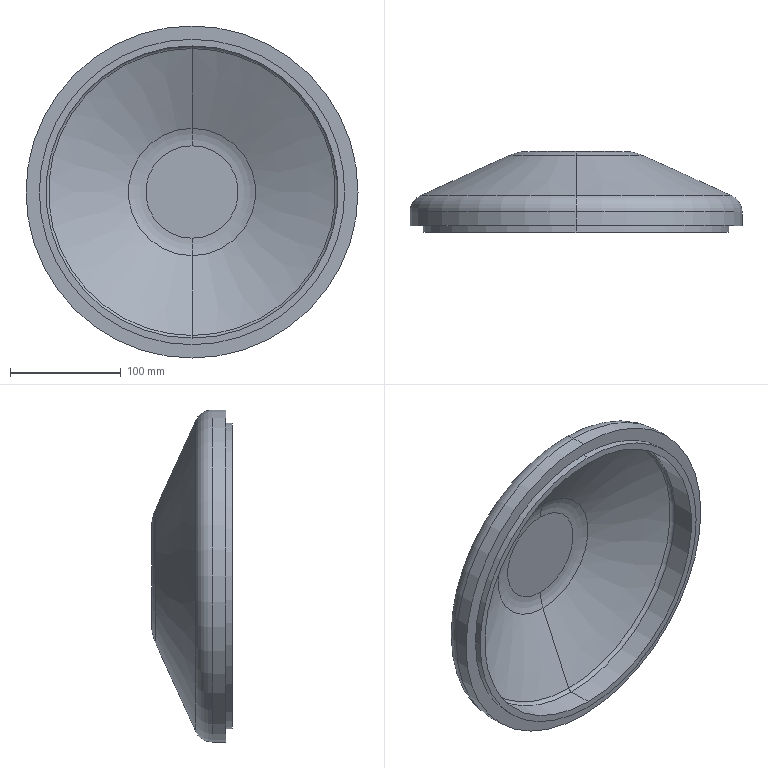Part | SolidWorks | features Fillet 4, Revolution 1 | 1 solid | 22 faces | box 300 x 73 x 300 mm | volume 1152181 mm3 | torus 8 | cylinder 6 | cone 4 | plane 4 | commonest cylinder face diameters 264 x2 276 x2 300 x2
STEP:
#1=CARTESIAN_POINT('',(0.,20.241,129.655));
#2=VERTEX_POINT('',#1);
#3=CARTESIAN_POINT('',(0.,20.241,-129.655));
#4=VERTEX_POINT('',#3);
#5=CARTESIAN_POINT('',(0.,20.241,0.));
#6=DIRECTION('',(0.,-1.,0.));
#7=DIRECTION('',(0.,0.,-1.));
#8=AXIS2_PLACEMENT_3D('',#5,#6,#7);
#9=CIRCLE('',#8,129.655);
#10=EDGE_CURVE('',#2,#4,#9,.T.);
#11=ORIENTED_EDGE('',*,*,#10,.F.);
#12=CARTESIAN_POINT('',(0.,16.6,132.));
#13=VERTEX_POINT('',#12);
#14=CARTESIAN_POINT('',(0.,16.6,128.));
#15=DIRECTION('',(1.,0.,0.));
#16=DIRECTION('',(0.,0.,-1.));
#17=AXIS2_PLACEMENT_3D('',#14,#15,#16);
#18=CIRCLE('',#17,4.);
#19=EDGE_CURVE('',#2,#13,#18,.T.);
#20=ORIENTED_EDGE('',*,*,#19,.T.);
#21=CARTESIAN_POINT('',(0.,16.6,-132.));
#22=VERTEX_POINT('',#21);
#23=CARTESIAN_POINT('',(0.,16.6,0.));
#24=DIRECTION('',(0.,1.,0.));
#25=DIRECTION('',(0.,0.,-1.));
#26=AXIS2_PLACEMENT_3D('',#23,#24,#25);
#27=CIRCLE('',#26,132.);
#28=EDGE_CURVE('',#22,#13,#27,.T.);
#29=ORIENTED_EDGE('',*,*,#28,.F.);
#30=CARTESIAN_POINT('',(0.,16.6,-128.));
#31=DIRECTION('',(-1.,0.,0.));
#32=DIRECTION('',(0.,0.,1.));
#33=AXIS2_PLACEMENT_3D('',#30,#31,#32);
#34=CIRCLE('',#33,4.);
#35=EDGE_CURVE('',#4,#22,#34,.T.);
#36=ORIENTED_EDGE('',*,*,#35,.F.);
#37=EDGE_LOOP('',(#11,#20,#29,#36));
#38=FACE_OUTER_BOUND('',#37,.T.);
#39=CARTESIAN_POINT('',(0.,16.6,0.));
#40=DIRECTION('',(0.,-1.,0.));
#41=DIRECTION('',(0.,0.,-1.));
#42=AXIS2_PLACEMENT_3D('',#39,#40,#41);
#43=TOROIDAL_SURFACE('',#42,128.,4.);
#44=ADVANCED_FACE('',(#38),#43,.F.);
#45=CARTESIAN_POINT('',(0.,13.872,-150.));
#46=VERTEX_POINT('',#45);
#47=CARTESIAN_POINT('',(0.,13.872,150.));
#48=VERTEX_POINT('',#47);
#49=CARTESIAN_POINT('',(0.,13.872,0.));
#50=DIRECTION('',(0.,-1.,0.));
#51=DIRECTION('',(0.,0.,1.));
#52=AXIS2_PLACEMENT_3D('',#49,#50,#51);
#53=CIRCLE('',#52,150.);
#54=EDGE_CURVE('',#46,#48,#53,.T.);
#55=ORIENTED_EDGE('',*,*,#54,.F.);
#56=CARTESIAN_POINT('',(0.,28.438,-140.621));
#57=VERTEX_POINT('',#56);
#58=CARTESIAN_POINT('',(0.,13.872,-134.));
#59=DIRECTION('',(1.,0.,0.));
#60=DIRECTION('',(0.,0.,-1.));
#61=AXIS2_PLACEMENT_3D('',#58,#59,#60);
#62=CIRCLE('',#61,16.);
#63=EDGE_CURVE('',#46,#57,#62,.T.);
#64=ORIENTED_EDGE('',*,*,#63,.T.);
#65=CARTESIAN_POINT('',(0.,28.438,140.621));
#66=VERTEX_POINT('',#65);
#67=CARTESIAN_POINT('',(0.,28.438,0.));
#68=DIRECTION('',(0.,1.,0.));
#69=DIRECTION('',(0.,0.,1.));
#70=AXIS2_PLACEMENT_3D('',#67,#68,#69);
#71=CIRCLE('',#70,140.621);
#72=EDGE_CURVE('',#66,#57,#71,.T.);
#73=ORIENTED_EDGE('',*,*,#72,.F.);
#74=CARTESIAN_POINT('',(0.,13.872,134.));
#75=DIRECTION('',(-1.,0.,0.));
#76=DIRECTION('',(0.,0.,1.));
#77=AXIS2_PLACEMENT_3D('',#74,#75,#76);
#78=CIRCLE('',#77,16.);
#79=EDGE_CURVE('',#48,#66,#78,.T.);
#80=ORIENTED_EDGE('',*,*,#79,.F.);
#81=EDGE_LOOP('',(#55,#64,#73,#80));
#82=FACE_OUTER_BOUND('',#81,.T.);
#83=CARTESIAN_POINT('',(0.,13.872,0.));
#84=DIRECTION('',(0.,1.,0.));
#85=DIRECTION('',(0.,0.,1.));
#86=AXIS2_PLACEMENT_3D('',#83,#84,#85);
#87=TOROIDAL_SURFACE('',#86,134.,16.);
#88=ADVANCED_FACE('',(#82),#87,.T.);
#89=CARTESIAN_POINT('',(0.,53.042,-57.493));
#90=VERTEX_POINT('',#89);
#91=CARTESIAN_POINT('',(0.,53.042,57.493));
#92=VERTEX_POINT('',#91);
#93=CARTESIAN_POINT('',(0.,53.042,0.));
#94=DIRECTION('',(0.,1.,0.));
#95=DIRECTION('',(0.,0.,-1.));
#96=AXIS2_PLACEMENT_3D('',#93,#94,#95);
#97=CIRCLE('',#96,57.493);
#98=EDGE_CURVE('',#90,#92,#97,.T.);
#99=ORIENTED_EDGE('',*,*,#98,.F.);
#100=CARTESIAN_POINT('',(0.,56.448,-41.769));
#101=VERTEX_POINT('',#100);
#102=CARTESIAN_POINT('',(0.,18.448,-41.769));
#103=DIRECTION('',(1.,0.,0.));
#104=DIRECTION('',(0.,0.,-1.));
#105=AXIS2_PLACEMENT_3D('',#102,#103,#104);
#106=CIRCLE('',#105,38.);
#107=EDGE_CURVE('',#90,#101,#106,.T.);
#108=ORIENTED_EDGE('',*,*,#107,.T.);
#109=CARTESIAN_POINT('',(0.,56.448,41.769));
#110=VERTEX_POINT('',#109);
#111=CARTESIAN_POINT('',(0.,56.448,0.));
#112=DIRECTION('',(0.,-1.,0.));
#113=DIRECTION('',(0.,0.,1.));
#114=AXIS2_PLACEMENT_3D('',#111,#112,#113);
#115=CIRCLE('',#114,41.769);
#116=EDGE_CURVE('',#110,#101,#115,.T.);
#117=ORIENTED_EDGE('',*,*,#116,.F.);
#118=CARTESIAN_POINT('',(0.,18.448,41.769));
#119=DIRECTION('',(-1.,0.,0.));
#120=DIRECTION('',(0.,0.,1.));
#121=AXIS2_PLACEMENT_3D('',#118,#119,#120);
#122=CIRCLE('',#121,38.);
#123=EDGE_CURVE('',#92,#110,#122,.T.);
#124=ORIENTED_EDGE('',*,*,#123,.F.);
#125=EDGE_LOOP('',(#99,#108,#117,#124));
#126=FACE_OUTER_BOUND('',#125,.T.);
#127=CARTESIAN_POINT('',(0.,18.448,0.));
#128=DIRECTION('',(0.,1.,0.));
#129=DIRECTION('',(0.,0.,1.));
#130=AXIS2_PLACEMENT_3D('',#127,#128,#129);
#131=TOROIDAL_SURFACE('',#130,41.769,38.);
#132=ADVANCED_FACE('',(#126),#131,.F.);
#133=CARTESIAN_POINT('',(0.,68.448,43.935));
#134=VERTEX_POINT('',#133);
#135=CARTESIAN_POINT('',(0.,68.448,-43.935));
#136=VERTEX_POINT('',#135);
#137=CARTESIAN_POINT('',(0.,68.448,0.));
#138=DIRECTION('',(0.,1.,0.));
#139=DIRECTION('',(0.,0.,-1.));
#140=AXIS2_PLACEMENT_3D('',#137,#138,#139);
#141=CIRCLE('',#140,43.935);
#142=EDGE_CURVE('',#134,#136,#141,.T.);
#143=ORIENTED_EDGE('',*,*,#142,.F.);
#144=CARTESIAN_POINT('',(0.,64.863,60.487));
#145=VERTEX_POINT('',#144);
#146=CARTESIAN_POINT('',(0.,28.448,43.935));
#147=DIRECTION('',(1.,0.,0.));
#148=DIRECTION('',(0.,0.,-1.));
#149=AXIS2_PLACEMENT_3D('',#146,#147,#148);
#150=CIRCLE('',#149,40.);
#151=EDGE_CURVE('',#134,#145,#150,.T.);
#152=ORIENTED_EDGE('',*,*,#151,.T.);
#153=CARTESIAN_POINT('',(0.,64.863,-60.487));
#154=VERTEX_POINT('',#153);
#155=CARTESIAN_POINT('',(0.,64.863,0.));
#156=DIRECTION('',(0.,-1.,0.));
#157=DIRECTION('',(0.,0.,1.));
#158=AXIS2_PLACEMENT_3D('',#155,#156,#157);
#159=CIRCLE('',#158,60.487);
#160=EDGE_CURVE('',#154,#145,#159,.T.);
#161=ORIENTED_EDGE('',*,*,#160,.F.);
#162=CARTESIAN_POINT('',(0.,28.448,-43.935));
#163=DIRECTION('',(-1.,0.,0.));
#164=DIRECTION('',(0.,0.,1.));
#165=AXIS2_PLACEMENT_3D('',#162,#163,#164);
#166=CIRCLE('',#165,40.);
#167=EDGE_CURVE('',#136,#154,#166,.T.);
#168=ORIENTED_EDGE('',*,*,#167,.F.);
#169=EDGE_LOOP('',(#143,#152,#161,#168));
#170=FACE_OUTER_BOUND('',#169,.T.);
#171=CARTESIAN_POINT('',(0.,28.448,0.));
#172=DIRECTION('',(0.,-1.,0.));
#173=DIRECTION('',(0.,0.,-1.));
#174=AXIS2_PLACEMENT_3D('',#171,#172,#173);
#175=TOROIDAL_SURFACE('',#174,43.935,40.);
#176=ADVANCED_FACE('',(#170),#175,.T.);
#177=CARTESIAN_POINT('',(0.,1.448,-138.));
#178=VERTEX_POINT('',#177);
#179=CARTESIAN_POINT('',(0.,1.448,138.));
#180=VERTEX_POINT('',#179);
#181=CARTESIAN_POINT('',(0.,1.448,0.));
#182=DIRECTION('',(0.,-1.,0.));
#183=DIRECTION('',(0.,0.,-1.));
#184=AXIS2_PLACEMENT_3D('',#181,#182,#183);
#185=CIRCLE('',#184,138.);
#186=EDGE_CURVE('',#178,#180,#185,.T.);
#187=ORIENTED_EDGE('',*,*,#186,.T.);
#188=CARTESIAN_POINT('',(0.,-4.552,138.));
#189=VERTEX_POINT('',#188);
#190=CARTESIAN_POINT('',(0.,0.,138.));
#191=DIRECTION('',(0.,-1.,0.));
#192=VECTOR('',#191,1000.);
#193=LINE('',#190,#192);
#194=EDGE_CURVE('',#180,#189,#193,.T.);
#195=ORIENTED_EDGE('',*,*,#194,.T.);
#196=CARTESIAN_POINT('',(0.,-4.552,-138.));
#197=VERTEX_POINT('',#196);
#198=CARTESIAN_POINT('',(0.,-4.552,0.));
#199=DIRECTION('',(0.,-1.,0.));
#200=DIRECTION('',(0.,0.,-1.));
#201=AXIS2_PLACEMENT_3D('',#198,#199,#200);
#202=CIRCLE('',#201,138.);
#203=EDGE_CURVE('',#197,#189,#202,.T.);
#204=ORIENTED_EDGE('',*,*,#203,.F.);
#205=CARTESIAN_POINT('',(0.,0.,-138.));
#206=DIRECTION('',(0.,-1.,0.));
#207=VECTOR('',#206,1000.);
#208=LINE('',#205,#207);
#209=EDGE_CURVE('',#178,#197,#208,.T.);
#210=ORIENTED_EDGE('',*,*,#209,.F.);
#211=EDGE_LOOP('',(#187,#195,#204,#210));
#212=FACE_OUTER_BOUND('',#211,.T.);
#213=CARTESIAN_POINT('',(0.,0.,0.));
#214=DIRECTION('',(0.,-1.,0.));
#215=DIRECTION('',(0.,0.,-1.));
#216=AXIS2_PLACEMENT_3D('',#213,#214,#215);
#217=CYLINDRICAL_SURFACE('',#216,138.);
#218=ADVANCED_FACE('',(#212),#217,.T.);
#219=ORIENTED_EDGE('',*,*,#28,.T.);
#220=CARTESIAN_POINT('',(0.,-4.552,132.));
#221=VERTEX_POINT('',#220);
#222=CARTESIAN_POINT('',(0.,0.,132.));
#223=DIRECTION('',(0.,-1.,0.));
#224=VECTOR('',#223,1000.);
#225=LINE('',#222,#224);
#226=EDGE_CURVE('',#13,#221,#225,.T.);
#227=ORIENTED_EDGE('',*,*,#226,.T.);
#228=CARTESIAN_POINT('',(0.,-4.552,-132.));
#229=VERTEX_POINT('',#228);
#230=CARTESIAN_POINT('',(0.,-4.552,0.));
#231=DIRECTION('',(0.,-1.,0.));
#232=DIRECTION('',(0.,0.,-1.));
#233=AXIS2_PLACEMENT_3D('',#230,#231,#232);
#234=CIRCLE('',#233,132.);
#235=EDGE_CURVE('',#221,#229,#234,.T.);
#236=ORIENTED_EDGE('',*,*,#235,.T.);
#237=CARTESIAN_POINT('',(0.,0.,-132.));
#238=DIRECTION('',(0.,-1.,0.));
#239=VECTOR('',#238,1000.);
#240=LINE('',#237,#239);
#241=EDGE_CURVE('',#22,#229,#240,.T.);
#242=ORIENTED_EDGE('',*,*,#241,.F.);
#243=EDGE_LOOP('',(#219,#227,#236,#242));
#244=FACE_OUTER_BOUND('',#243,.T.);
#245=CARTESIAN_POINT('',(0.,0.,0.));
#246=DIRECTION('',(0.,-1.,0.));
#247=DIRECTION('',(0.,0.,-1.));
#248=AXIS2_PLACEMENT_3D('',#245,#246,#247);
#249=CYLINDRICAL_SURFACE('',#248,132.);
#250=ADVANCED_FACE('',(#244),#249,.F.);
#251=ORIENTED_EDGE('',*,*,#98,.T.);
#252=CARTESIAN_POINT('',(0.,19.175,132.));
#253=DIRECTION('',(0.,-0.4138,0.9104));
#254=VECTOR('',#253,1000.);
#255=LINE('',#252,#254);
#256=EDGE_CURVE('',#92,#2,#255,.T.);
#257=ORIENTED_EDGE('',*,*,#256,.T.);
#258=ORIENTED_EDGE('',*,*,#10,.T.);
#259=CARTESIAN_POINT('',(0.,19.175,-132.));
#260=DIRECTION('',(0.,-0.4138,-0.9104));
#261=VECTOR('',#260,1000.);
#262=LINE('',#259,#261);
#263=EDGE_CURVE('',#90,#4,#262,.T.);
#264=ORIENTED_EDGE('',*,*,#263,.F.);
#265=EDGE_LOOP('',(#251,#257,#258,#264));
#266=FACE_OUTER_BOUND('',#265,.T.);
#267=CARTESIAN_POINT('',(0.,19.175,0.));
#268=DIRECTION('',(0.,-1.,0.));
#269=DIRECTION('',(0.,0.,-1.));
#270=AXIS2_PLACEMENT_3D('',#267,#268,#269);
#271=CONICAL_SURFACE('',#270,132.,1.144);
#272=ADVANCED_FACE('',(#266),#271,.F.);
#273=ORIENTED_EDGE('',*,*,#160,.T.);
#274=CARTESIAN_POINT('',(0.,68.448,52.599));
#275=DIRECTION('',(0.,-0.4138,0.9104));
#276=VECTOR('',#275,1000.);
#277=LINE('',#274,#276);
#278=EDGE_CURVE('',#145,#66,#277,.T.);
#279=ORIENTED_EDGE('',*,*,#278,.T.);
#280=ORIENTED_EDGE('',*,*,#72,.T.);
#281=CARTESIAN_POINT('',(0.,68.448,-52.599));
#282=DIRECTION('',(0.,-0.4138,-0.9104));
#283=VECTOR('',#282,1000.);
#284=LINE('',#281,#283);
#285=EDGE_CURVE('',#154,#57,#284,.T.);
#286=ORIENTED_EDGE('',*,*,#285,.F.);
#287=EDGE_LOOP('',(#273,#279,#280,#286));
#288=FACE_OUTER_BOUND('',#287,.T.);
#289=CARTESIAN_POINT('',(0.,68.448,0.));
#290=DIRECTION('',(0.,-1.,0.));
#291=DIRECTION('',(0.,0.,-1.));
#292=AXIS2_PLACEMENT_3D('',#289,#290,#291);
#293=CONICAL_SURFACE('',#292,52.599,1.144);
#294=ADVANCED_FACE('',(#288),#293,.T.);
#295=ORIENTED_EDGE('',*,*,#54,.T.);
#296=CARTESIAN_POINT('',(0.,1.448,150.));
#297=VERTEX_POINT('',#296);
#298=CARTESIAN_POINT('',(0.,0.,150.));
#299=DIRECTION('',(0.,-1.,0.));
#300=VECTOR('',#299,1000.);
#301=LINE('',#298,#300);
#302=EDGE_CURVE('',#48,#297,#301,.T.);
#303=ORIENTED_EDGE('',*,*,#302,.T.);
#304=CARTESIAN_POINT('',(0.,1.448,-150.));
#305=VERTEX_POINT('',#304);
#306=CARTESIAN_POINT('',(0.,1.448,0.));
#307=DIRECTION('',(0.,-1.,0.));
#308=DIRECTION('',(0.,0.,-1.));
#309=AXIS2_PLACEMENT_3D('',#306,#307,#308);
#310=CIRCLE('',#309,150.);
#311=EDGE_CURVE('',#305,#297,#310,.T.);
#312=ORIENTED_EDGE('',*,*,#311,.F.);
#313=CARTESIAN_POINT('',(0.,0.,-150.));
#314=DIRECTION('',(0.,-1.,0.));
#315=VECTOR('',#314,1000.);
#316=LINE('',#313,#315);
#317=EDGE_CURVE('',#46,#305,#316,.T.);
#318=ORIENTED_EDGE('',*,*,#317,.F.);
#319=EDGE_LOOP('',(#295,#303,#312,#318));
#320=FACE_OUTER_BOUND('',#319,.T.);
#321=CARTESIAN_POINT('',(0.,0.,0.));
#322=DIRECTION('',(0.,-1.,0.));
#323=DIRECTION('',(0.,0.,-1.));
#324=AXIS2_PLACEMENT_3D('',#321,#322,#323);
#325=CYLINDRICAL_SURFACE('',#324,150.);
#326=ADVANCED_FACE('',(#320),#325,.T.);
#327=ORIENTED_EDGE('',*,*,#186,.F.);
#328=CARTESIAN_POINT('',(0.,1.448,0.));
#329=DIRECTION('',(0.,-1.,0.));
#330=DIRECTION('',(0.,0.,-1.));
#331=AXIS2_PLACEMENT_3D('',#328,#329,#330);
#332=CIRCLE('',#331,138.);
#333=EDGE_CURVE('',#180,#178,#332,.T.);
#334=ORIENTED_EDGE('',*,*,#333,.F.);
#335=EDGE_LOOP('',(#327,#334));
#336=FACE_BOUND('',#335,.T.);
#337=ORIENTED_EDGE('',*,*,#311,.T.);
#338=CARTESIAN_POINT('',(0.,1.448,0.));
#339=DIRECTION('',(0.,-1.,0.));
#340=DIRECTION('',(0.,0.,-1.));
#341=AXIS2_PLACEMENT_3D('',#338,#339,#340);
#342=CIRCLE('',#341,150.);
#343=EDGE_CURVE('',#297,#305,#342,.T.);
#344=ORIENTED_EDGE('',*,*,#343,.T.);
#345=EDGE_LOOP('',(#337,#344));
#346=FACE_OUTER_BOUND('',#345,.T.);
#347=CARTESIAN_POINT('',(-150.,1.448,0.));
#348=DIRECTION('',(0.,1.,0.));
#349=DIRECTION('',(0.,0.,1.));
#350=AXIS2_PLACEMENT_3D('',#347,#348,#349);
#351=PLANE('',#350);
#352=ADVANCED_FACE('',(#336,#346),#351,.F.);
#353=ORIENTED_EDGE('',*,*,#302,.F.);
#354=CARTESIAN_POINT('',(0.,13.872,0.));
#355=DIRECTION('',(0.,-1.,0.));
#356=DIRECTION('',(0.,0.,1.));
#357=AXIS2_PLACEMENT_3D('',#354,#355,#356);
#358=CIRCLE('',#357,150.);
#359=EDGE_CURVE('',#48,#46,#358,.T.);
#360=ORIENTED_EDGE('',*,*,#359,.T.);
#361=ORIENTED_EDGE('',*,*,#317,.T.);
#362=ORIENTED_EDGE('',*,*,#343,.F.);
#363=EDGE_LOOP('',(#353,#360,#361,#362));
#364=FACE_OUTER_BOUND('',#363,.T.);
#365=CARTESIAN_POINT('',(0.,0.,0.));
#366=DIRECTION('',(0.,-1.,0.));
#367=DIRECTION('',(0.,0.,-1.));
#368=AXIS2_PLACEMENT_3D('',#365,#366,#367);
#369=CYLINDRICAL_SURFACE('',#368,150.);
#370=ADVANCED_FACE('',(#364),#369,.T.);
#371=ORIENTED_EDGE('',*,*,#278,.F.);
#372=CARTESIAN_POINT('',(0.,64.863,0.));
#373=DIRECTION('',(0.,-1.,0.));
#374=DIRECTION('',(0.,0.,1.));
#375=AXIS2_PLACEMENT_3D('',#372,#373,#374);
#376=CIRCLE('',#375,60.487);
#377=EDGE_CURVE('',#145,#154,#376,.T.);
#378=ORIENTED_EDGE('',*,*,#377,.T.);
#379=ORIENTED_EDGE('',*,*,#285,.T.);
#380=CARTESIAN_POINT('',(0.,28.438,0.));
#381=DIRECTION('',(0.,1.,0.));
#382=DIRECTION('',(0.,0.,1.));
#383=AXIS2_PLACEMENT_3D('',#380,#381,#382);
#384=CIRCLE('',#383,140.621);
#385=EDGE_CURVE('',#57,#66,#384,.T.);
#386=ORIENTED_EDGE('',*,*,#385,.T.);
#387=EDGE_LOOP('',(#371,#378,#379,#386));
#388=FACE_OUTER_BOUND('',#387,.T.);
#389=CARTESIAN_POINT('',(0.,68.448,0.));
#390=DIRECTION('',(0.,-1.,0.));
#391=DIRECTION('',(0.,0.,-1.));
#392=AXIS2_PLACEMENT_3D('',#389,#390,#391);
#393=CONICAL_SURFACE('',#392,52.599,1.144);
#394=ADVANCED_FACE('',(#388),#393,.T.);
#395=CARTESIAN_POINT('',(0.,68.448,0.));
#396=DIRECTION('',(0.,1.,0.));
#397=DIRECTION('',(0.,0.,-1.));
#398=AXIS2_PLACEMENT_3D('',#395,#396,#397);
#399=CIRCLE('',#398,43.935);
#400=EDGE_CURVE('',#136,#134,#399,.T.);
#401=ORIENTED_EDGE('',*,*,#400,.T.);
#402=ORIENTED_EDGE('',*,*,#142,.T.);
#403=EDGE_LOOP('',(#401,#402));
#404=FACE_OUTER_BOUND('',#403,.T.);
#405=CARTESIAN_POINT('',(-52.599,68.448,0.));
#406=DIRECTION('',(0.,-1.,0.));
#407=DIRECTION('',(0.,0.,-1.));
#408=AXIS2_PLACEMENT_3D('',#405,#406,#407);
#409=PLANE('',#408);
#410=ADVANCED_FACE('',(#404),#409,.F.);
#411=ORIENTED_EDGE('',*,*,#116,.T.);
#412=CARTESIAN_POINT('',(0.,56.448,0.));
#413=DIRECTION('',(0.,-1.,0.));
#414=DIRECTION('',(0.,0.,1.));
#415=AXIS2_PLACEMENT_3D('',#412,#413,#414);
#416=CIRCLE('',#415,41.769);
#417=EDGE_CURVE('',#101,#110,#416,.T.);
#418=ORIENTED_EDGE('',*,*,#417,.T.);
#419=EDGE_LOOP('',(#411,#418));
#420=FACE_OUTER_BOUND('',#419,.T.);
#421=CARTESIAN_POINT('',(-50.,56.448,0.));
#422=DIRECTION('',(0.,1.,0.));
#423=DIRECTION('',(0.,0.,1.));
#424=AXIS2_PLACEMENT_3D('',#421,#422,#423);
#425=PLANE('',#424);
#426=ADVANCED_FACE('',(#420),#425,.F.);
#427=ORIENTED_EDGE('',*,*,#256,.F.);
#428=CARTESIAN_POINT('',(0.,53.042,0.));
#429=DIRECTION('',(0.,1.,0.));
#430=DIRECTION('',(0.,0.,-1.));
#431=AXIS2_PLACEMENT_3D('',#428,#429,#430);
#432=CIRCLE('',#431,57.493);
#433=EDGE_CURVE('',#92,#90,#432,.T.);
#434=ORIENTED_EDGE('',*,*,#433,.T.);
#435=ORIENTED_EDGE('',*,*,#263,.T.);
#436=CARTESIAN_POINT('',(0.,20.241,0.));
#437=DIRECTION('',(0.,-1.,0.));
#438=DIRECTION('',(0.,0.,-1.));
#439=AXIS2_PLACEMENT_3D('',#436,#437,#438);
#440=CIRCLE('',#439,129.655);
#441=EDGE_CURVE('',#4,#2,#440,.T.);
#442=ORIENTED_EDGE('',*,*,#441,.T.);
#443=EDGE_LOOP('',(#427,#434,#435,#442));
#444=FACE_OUTER_BOUND('',#443,.T.);
#445=CARTESIAN_POINT('',(0.,19.175,0.));
#446=DIRECTION('',(0.,-1.,0.));
#447=DIRECTION('',(0.,0.,-1.));
#448=AXIS2_PLACEMENT_3D('',#445,#446,#447);
#449=CONICAL_SURFACE('',#448,132.,1.144);
#450=ADVANCED_FACE('',(#444),#449,.F.);
#451=ORIENTED_EDGE('',*,*,#226,.F.);
#452=CARTESIAN_POINT('',(0.,16.6,0.));
#453=DIRECTION('',(0.,1.,0.));
#454=DIRECTION('',(0.,0.,-1.));
#455=AXIS2_PLACEMENT_3D('',#452,#453,#454);
#456=CIRCLE('',#455,132.);
#457=EDGE_CURVE('',#13,#22,#456,.T.);
#458=ORIENTED_EDGE('',*,*,#457,.T.);
#459=ORIENTED_EDGE('',*,*,#241,.T.);
#460=CARTESIAN_POINT('',(0.,-4.552,0.));
#461=DIRECTION('',(0.,-1.,0.));
#462=DIRECTION('',(0.,0.,-1.));
#463=AXIS2_PLACEMENT_3D('',#460,#461,#462);
#464=CIRCLE('',#463,132.);
#465=EDGE_CURVE('',#229,#221,#464,.T.);
#466=ORIENTED_EDGE('',*,*,#465,.T.);
#467=EDGE_LOOP('',(#451,#458,#459,#466));
#468=FACE_OUTER_BOUND('',#467,.T.);
#469=CARTESIAN_POINT('',(0.,0.,0.));
#470=DIRECTION('',(0.,-1.,0.));
#471=DIRECTION('',(0.,0.,-1.));
#472=AXIS2_PLACEMENT_3D('',#469,#470,#471);
#473=CYLINDRICAL_SURFACE('',#472,132.);
#474=ADVANCED_FACE('',(#468),#473,.F.);
#475=ORIENTED_EDGE('',*,*,#465,.F.);
#476=ORIENTED_EDGE('',*,*,#235,.F.);
#477=EDGE_LOOP('',(#475,#476));
#478=FACE_BOUND('',#477,.T.);
#479=ORIENTED_EDGE('',*,*,#203,.T.);
#480=CARTESIAN_POINT('',(0.,-4.552,0.));
#481=DIRECTION('',(0.,-1.,0.));
#482=DIRECTION('',(0.,0.,-1.));
#483=AXIS2_PLACEMENT_3D('',#480,#481,#482);
#484=CIRCLE('',#483,138.);
#485=EDGE_CURVE('',#189,#197,#484,.T.);
#486=ORIENTED_EDGE('',*,*,#485,.T.);
#487=EDGE_LOOP('',(#479,#486));
#488=FACE_OUTER_BOUND('',#487,.T.);
#489=CARTESIAN_POINT('',(-138.,-4.552,0.));
#490=DIRECTION('',(0.,1.,0.));
#491=DIRECTION('',(0.,0.,1.));
#492=AXIS2_PLACEMENT_3D('',#489,#490,#491);
#493=PLANE('',#492);
#494=ADVANCED_FACE('',(#478,#488),#493,.F.);
#495=ORIENTED_EDGE('',*,*,#194,.F.);
#496=ORIENTED_EDGE('',*,*,#333,.T.);
#497=ORIENTED_EDGE('',*,*,#209,.T.);
#498=ORIENTED_EDGE('',*,*,#485,.F.);
#499=EDGE_LOOP('',(#495,#496,#497,#498));
#500=FACE_OUTER_BOUND('',#499,.T.);
#501=CARTESIAN_POINT('',(0.,0.,0.));
#502=DIRECTION('',(0.,-1.,0.));
#503=DIRECTION('',(0.,0.,-1.));
#504=AXIS2_PLACEMENT_3D('',#501,#502,#503);
#505=CYLINDRICAL_SURFACE('',#504,138.);
#506=ADVANCED_FACE('',(#500),#505,.T.);
#507=ORIENTED_EDGE('',*,*,#151,.F.);
#508=ORIENTED_EDGE('',*,*,#400,.F.);
#509=ORIENTED_EDGE('',*,*,#167,.T.);
#510=ORIENTED_EDGE('',*,*,#377,.F.);
#511=EDGE_LOOP('',(#507,#508,#509,#510));
#512=FACE_OUTER_BOUND('',#511,.T.);
#513=CARTESIAN_POINT('',(0.,28.448,0.));
#514=DIRECTION('',(0.,-1.,0.));
#515=DIRECTION('',(0.,0.,-1.));
#516=AXIS2_PLACEMENT_3D('',#513,#514,#515);
#517=TOROIDAL_SURFACE('',#516,43.935,40.);
#518=ADVANCED_FACE('',(#512),#517,.T.);
#519=ORIENTED_EDGE('',*,*,#107,.F.);
#520=ORIENTED_EDGE('',*,*,#433,.F.);
#521=ORIENTED_EDGE('',*,*,#123,.T.);
#522=ORIENTED_EDGE('',*,*,#417,.F.);
#523=EDGE_LOOP('',(#519,#520,#521,#522));
#524=FACE_OUTER_BOUND('',#523,.T.);
#525=CARTESIAN_POINT('',(0.,18.448,0.));
#526=DIRECTION('',(0.,1.,0.));
#527=DIRECTION('',(0.,0.,1.));
#528=AXIS2_PLACEMENT_3D('',#525,#526,#527);
#529=TOROIDAL_SURFACE('',#528,41.769,38.);
#530=ADVANCED_FACE('',(#524),#529,.F.);
#531=ORIENTED_EDGE('',*,*,#63,.F.);
#532=ORIENTED_EDGE('',*,*,#359,.F.);
#533=ORIENTED_EDGE('',*,*,#79,.T.);
#534=ORIENTED_EDGE('',*,*,#385,.F.);
#535=EDGE_LOOP('',(#531,#532,#533,#534));
#536=FACE_OUTER_BOUND('',#535,.T.);
#537=CARTESIAN_POINT('',(0.,13.872,0.));
#538=DIRECTION('',(0.,1.,0.));
#539=DIRECTION('',(0.,0.,1.));
#540=AXIS2_PLACEMENT_3D('',#537,#538,#539);
#541=TOROIDAL_SURFACE('',#540,134.,16.);
#542=ADVANCED_FACE('',(#536),#541,.T.);
#543=ORIENTED_EDGE('',*,*,#19,.F.);
#544=ORIENTED_EDGE('',*,*,#441,.F.);
#545=ORIENTED_EDGE('',*,*,#35,.T.);
#546=ORIENTED_EDGE('',*,*,#457,.F.);
#547=EDGE_LOOP('',(#543,#544,#545,#546));
#548=FACE_OUTER_BOUND('',#547,.T.);
#549=CARTESIAN_POINT('',(0.,16.6,0.));
#550=DIRECTION('',(0.,-1.,0.));
#551=DIRECTION('',(0.,0.,-1.));
#552=AXIS2_PLACEMENT_3D('',#549,#550,#551);
#553=TOROIDAL_SURFACE('',#552,128.,4.);
#554=ADVANCED_FACE('',(#548),#553,.F.);
#555=CLOSED_SHELL('',(#44,#88,#132,#176,#218,#250,#272,#294,#326,#352,#370,#394,#410,#426,#450,#474,#494,#506,#518,#530,#542,#554));
#556=MANIFOLD_SOLID_BREP('',#555);
#557=CARTESIAN_POINT('',(0.,0.,0.));
#558=DIRECTION('',(0.,0.,1.));
#559=DIRECTION('',(1.,0.,0.));
#560=AXIS2_PLACEMENT_3D('',#557,#558,#559);
#561=(LENGTH_UNIT()NAMED_UNIT(*)SI_UNIT(.MILLI.,.METRE.));
#562=UNCERTAINTY_MEASURE_WITH_UNIT(LENGTH_MEASURE(0.00001),#561,'','');
#563=(NAMED_UNIT(*)PLANE_ANGLE_UNIT()SI_UNIT($,.RADIAN.));
#564=(NAMED_UNIT(*)SI_UNIT($,.STERADIAN.)SOLID_ANGLE_UNIT());
#565=(GEOMETRIC_REPRESENTATION_CONTEXT(3)GLOBAL_UNCERTAINTY_ASSIGNED_CONTEXT((#562))GLOBAL_UNIT_ASSIGNED_CONTEXT((#561,#563,#564))REPRESENTATION_CONTEXT('',''));
#566=ADVANCED_BREP_SHAPE_REPRESENTATION('',(#556,#560),#565);